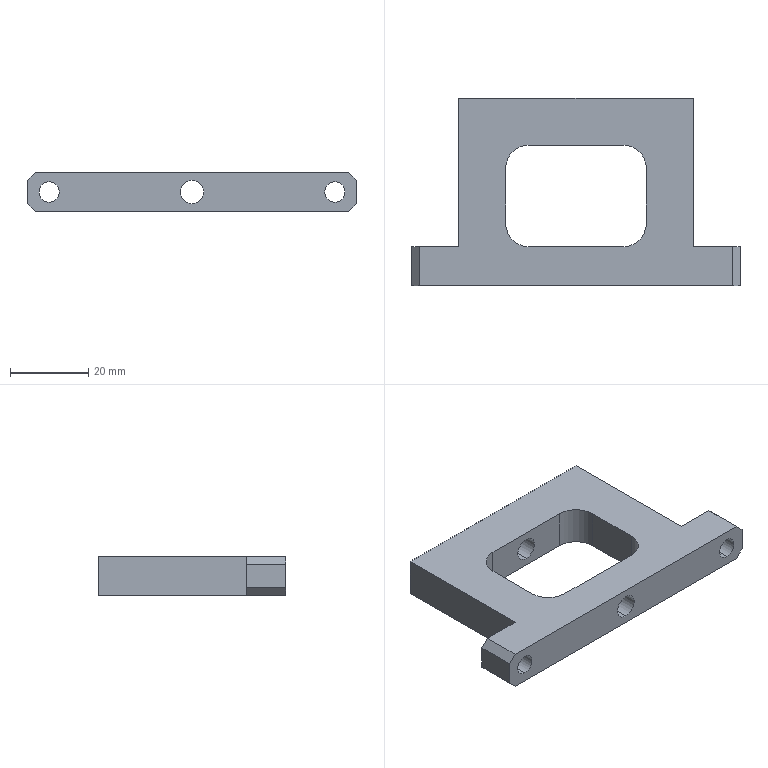Part | STEP file | QA-FB04 | 1 solid | 38 faces | box 84 x 48 x 10 mm | volume 20623 mm3 | plane 18 | cylinder 16 | cone 4 | commonest cylinder face diameters 4.2 x4 5.2 x4 6 x4 12 x4